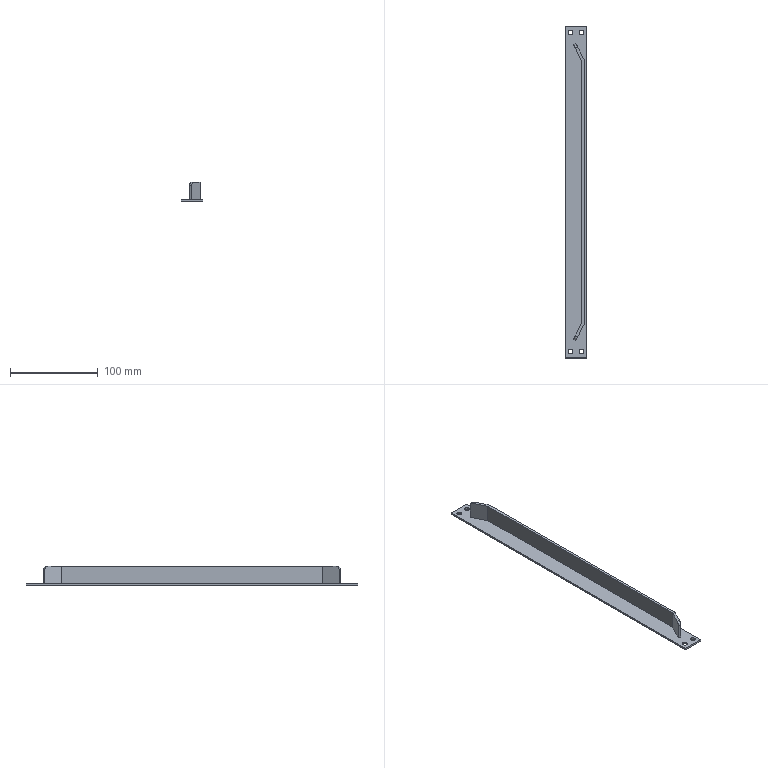Part | STEP file | blaszka 1 gietaV11 | 1 solid | 27 faces | box 24.5 x 378 x 22 mm | volume 38515 mm3 | plane 15 | cylinder 12 | commonest cylinder face diameters 5.5 x8 8 x2 12 x2